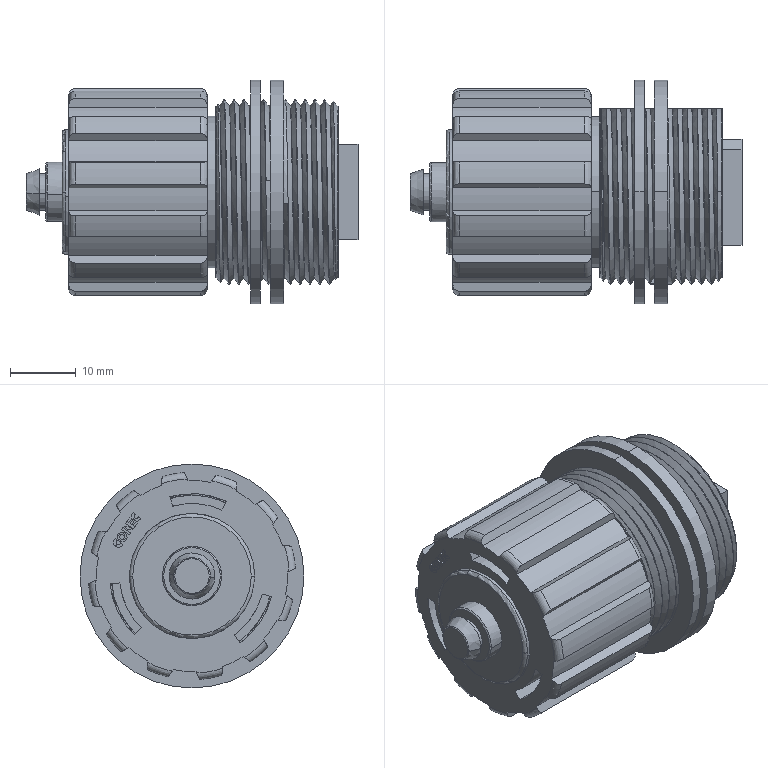Part | SolidWorks | features BaseBody 1 | 1 solid | 1436 faces | box 50.41 x 34 x 34 mm | volume 20764 mm3 | plane 891 | cylinder 331 | spline 162 | torus 40 | cone 12 | commonest cylinder face diameters 0.4 x56 28 x35 0.708 x28 1.494 x26 1 x20 1.6 x16